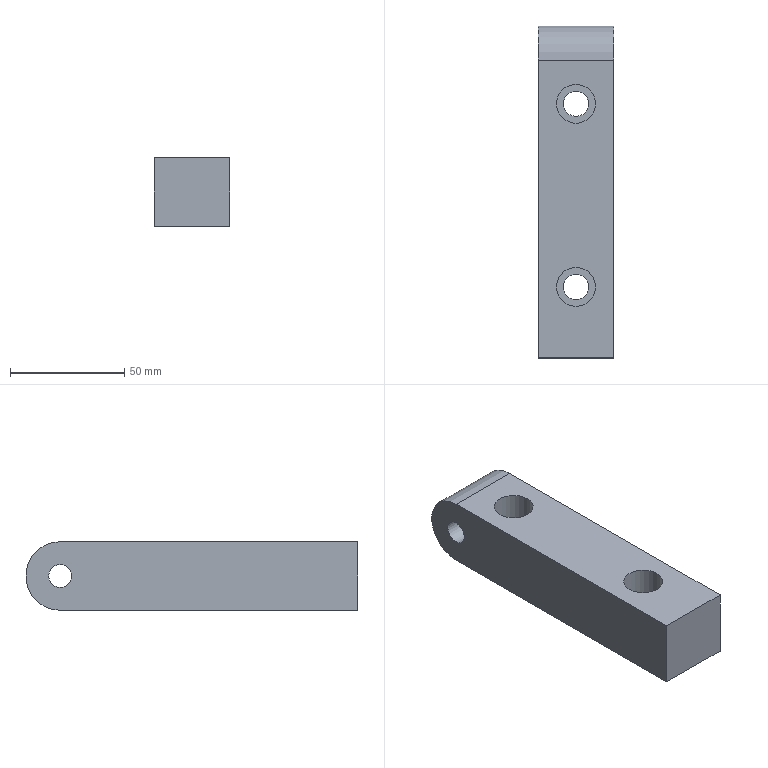Part | STEP file | gslz 2016.10.28-13_id1846_x_t | 1 solid | 13 faces | box 33 x 145.1 x 30 mm | volume 128184 mm3 | plane 7 | cylinder 6 | commonest cylinder face diameters 11 x2 17 x2 10.05 x1 30 x1
STEP:
#1=CARTESIAN_POINT('',(0.,0.,0.));
#2=DIRECTION('',(0.,0.,1.));
#3=DIRECTION('',(1.,0.,0.));
#4=AXIS2_PLACEMENT_3D('',#1,#2,#3);
#5=CARTESIAN_POINT('',(-1160.5,501.,-64.));
#6=VERTEX_POINT('',#5);
#7=CARTESIAN_POINT('',(-1171.5,501.,-64.));
#8=VERTEX_POINT('',#7);
#9=CARTESIAN_POINT('',(-1166.,501.,-64.));
#10=DIRECTION('',(0.,0.,1.));
#11=DIRECTION('',(-1.,0.,0.));
#12=AXIS2_PLACEMENT_3D('',#9,#10,#11);
#13=CIRCLE('',#12,5.5);
#14=CARTESIAN_POINT('',(-1166.,501.,-51.));
#15=DIRECTION('',(0.,0.,-1.));
#16=DIRECTION('',(0.,1.,0.));
#17=AXIS2_PLACEMENT_3D('',#14,#15,#16);
#18=CYLINDRICAL_SURFACE('',#17,5.5);
#19=CARTESIAN_POINT('',(10.996,13.));
#20=DIRECTION('',(-1.,0.));
#21=VECTOR('',#20,1.);
#22=LINE('',#19,#21);
#23=(GEOMETRIC_REPRESENTATION_CONTEXT(2)PARAMETRIC_REPRESENTATION_CONTEXT()REPRESENTATION_CONTEXT('',''));
#24=DEFINITIONAL_REPRESENTATION('',(#22),#23);
#25=PCURVE('',#18,#24);
#26=CARTESIAN_POINT('',(-1166.75,547.5,-64.));
#27=DIRECTION('',(0.,0.,1.));
#28=DIRECTION('',(-1.,0.,0.));
#29=AXIS2_PLACEMENT_3D('',#26,#27,#28);
#30=PLANE('',#29);
#31=CARTESIAN_POINT('',(-0.75,46.5));
#32=DIRECTION('',(1.,0.));
#33=AXIS2_PLACEMENT_2D('',#31,#32);
#34=CIRCLE('',#33,5.5);
#35=(GEOMETRIC_REPRESENTATION_CONTEXT(2)PARAMETRIC_REPRESENTATION_CONTEXT()REPRESENTATION_CONTEXT('',''));
#36=DEFINITIONAL_REPRESENTATION('',(#34),#35);
#37=PCURVE('',#30,#36);
#38=SURFACE_CURVE('',#13,(#25,#37),.PCURVE_S1.);
#39=EDGE_CURVE('',#6,#8,#38,.T.);
#40=ORIENTED_EDGE('',*,*,#39,.F.);
#41=CARTESIAN_POINT('',(-1160.5,501.,-79.));
#42=VERTEX_POINT('',#41);
#43=CARTESIAN_POINT('',(-1160.5,501.,-64.));
#44=CARTESIAN_POINT('',(-1160.5,501.,-79.));
#45=B_SPLINE_CURVE_WITH_KNOTS('',1,(#43,#44),.UNSPECIFIED.,.F.,.F.,(2,2),(13.,28.),.PIECEWISE_BEZIER_KNOTS.);
#46=CARTESIAN_POINT('',(7.854,0.));
#47=DIRECTION('',(0.,1.));
#48=VECTOR('',#47,1.);
#49=LINE('',#46,#48);
#50=(GEOMETRIC_REPRESENTATION_CONTEXT(2)PARAMETRIC_REPRESENTATION_CONTEXT()REPRESENTATION_CONTEXT('',''));
#51=DEFINITIONAL_REPRESENTATION('',(#49),#50);
#52=PCURVE('',#18,#51);
#53=CARTESIAN_POINT('',(1.571,0.));
#54=DIRECTION('',(0.,1.));
#55=VECTOR('',#54,1.);
#56=LINE('',#53,#55);
#57=(GEOMETRIC_REPRESENTATION_CONTEXT(2)PARAMETRIC_REPRESENTATION_CONTEXT()REPRESENTATION_CONTEXT('',''));
#58=DEFINITIONAL_REPRESENTATION('',(#56),#57);
#59=PCURVE('',#18,#58);
#60=SEAM_CURVE('',#45,(#52,#59),.PCURVE_S1.);
#61=EDGE_CURVE('',#6,#42,#60,.T.);
#62=ORIENTED_EDGE('',*,*,#61,.T.);
#63=CARTESIAN_POINT('',(-1166.,501.,-79.));
#64=DIRECTION('',(0.,0.,-1.));
#65=DIRECTION('',(1.,0.,0.));
#66=AXIS2_PLACEMENT_3D('',#63,#64,#65);
#67=CIRCLE('',#66,5.5);
#68=CARTESIAN_POINT('',(1.571,28.));
#69=DIRECTION('',(1.,0.));
#70=VECTOR('',#69,1.);
#71=LINE('',#68,#70);
#72=(GEOMETRIC_REPRESENTATION_CONTEXT(2)PARAMETRIC_REPRESENTATION_CONTEXT()REPRESENTATION_CONTEXT('',''));
#73=DEFINITIONAL_REPRESENTATION('',(#71),#72);
#74=PCURVE('',#18,#73);
#75=CARTESIAN_POINT('',(-1147.5,599.,-79.));
#76=DIRECTION('',(0.,0.,1.));
#77=DIRECTION('',(0.,-1.,0.));
#78=AXIS2_PLACEMENT_3D('',#75,#76,#77);
#79=PLANE('',#78);
#80=CARTESIAN_POINT('',(98.,-13.));
#81=CARTESIAN_POINT('',(107.526,-13.));
#82=CARTESIAN_POINT('',(102.763,-21.25));
#83=CARTESIAN_POINT('',(98.,-29.5));
#84=CARTESIAN_POINT('',(93.237,-21.25));
#85=CARTESIAN_POINT('',(88.474,-13.));
#86=CARTESIAN_POINT('',(98.,-13.));
#87=(BOUNDED_CURVE()B_SPLINE_CURVE(2,(#80,#81,#82,#83,#84,#85,#86),.UNSPECIFIED.,.T.,.F.)B_SPLINE_CURVE_WITH_KNOTS((1,2,2,2,2,1),(-2.094,0.,2.094,4.189,6.283,8.378),.UNSPECIFIED.)CURVE()GEOMETRIC_REPRESENTATION_ITEM()RATIONAL_B_SPLINE_CURVE((1.,0.5,1.,0.5,1.,0.5,1.))REPRESENTATION_ITEM(''));
#88=(GEOMETRIC_REPRESENTATION_CONTEXT(2)PARAMETRIC_REPRESENTATION_CONTEXT()REPRESENTATION_CONTEXT('',''));
#89=DEFINITIONAL_REPRESENTATION('',(#87),#88);
#90=PCURVE('',#79,#89);
#91=SURFACE_CURVE('',#67,(#74,#90),.PCURVE_S1.);
#92=EDGE_CURVE('',#42,#42,#91,.T.);
#93=ORIENTED_EDGE('',*,*,#92,.F.);
#94=ORIENTED_EDGE('',*,*,#61,.F.);
#95=CARTESIAN_POINT('',(-1166.,501.,-64.));
#96=DIRECTION('',(0.,0.,1.));
#97=DIRECTION('',(-1.,0.,0.));
#98=AXIS2_PLACEMENT_3D('',#95,#96,#97);
#99=CIRCLE('',#98,5.5);
#100=CARTESIAN_POINT('',(4.712,13.));
#101=DIRECTION('',(-1.,0.));
#102=VECTOR('',#101,1.);
#103=LINE('',#100,#102);
#104=(GEOMETRIC_REPRESENTATION_CONTEXT(2)PARAMETRIC_REPRESENTATION_CONTEXT()REPRESENTATION_CONTEXT('',''));
#105=DEFINITIONAL_REPRESENTATION('',(#103),#104);
#106=PCURVE('',#18,#105);
#107=CARTESIAN_POINT('',(-0.75,46.5));
#108=DIRECTION('',(1.,0.));
#109=AXIS2_PLACEMENT_2D('',#107,#108);
#110=CIRCLE('',#109,5.5);
#111=(GEOMETRIC_REPRESENTATION_CONTEXT(2)PARAMETRIC_REPRESENTATION_CONTEXT()REPRESENTATION_CONTEXT('',''));
#112=DEFINITIONAL_REPRESENTATION('',(#110),#111);
#113=PCURVE('',#30,#112);
#114=SURFACE_CURVE('',#99,(#106,#113),.PCURVE_S1.);
#115=EDGE_CURVE('',#8,#6,#114,.T.);
#116=ORIENTED_EDGE('',*,*,#115,.F.);
#117=EDGE_LOOP('',(#40,#62,#93,#94,#116));
#118=FACE_BOUND('',#117,.F.);
#119=ADVANCED_FACE('',(#118),#18,.F.);
#120=CARTESIAN_POINT('',(-1160.5,581.,-64.));
#121=VERTEX_POINT('',#120);
#122=CARTESIAN_POINT('',(-1171.5,581.,-64.));
#123=VERTEX_POINT('',#122);
#124=CARTESIAN_POINT('',(-1166.,581.,-64.));
#125=DIRECTION('',(0.,0.,1.));
#126=DIRECTION('',(-1.,0.,0.));
#127=AXIS2_PLACEMENT_3D('',#124,#125,#126);
#128=CIRCLE('',#127,5.5);
#129=CARTESIAN_POINT('',(-1166.,581.,-51.));
#130=DIRECTION('',(0.,0.,-1.));
#131=DIRECTION('',(0.,1.,0.));
#132=AXIS2_PLACEMENT_3D('',#129,#130,#131);
#133=CYLINDRICAL_SURFACE('',#132,5.5);
#134=CARTESIAN_POINT('',(10.996,13.));
#135=DIRECTION('',(-1.,0.));
#136=VECTOR('',#135,1.);
#137=LINE('',#134,#136);
#138=(GEOMETRIC_REPRESENTATION_CONTEXT(2)PARAMETRIC_REPRESENTATION_CONTEXT()REPRESENTATION_CONTEXT('',''));
#139=DEFINITIONAL_REPRESENTATION('',(#137),#138);
#140=PCURVE('',#133,#139);
#141=CARTESIAN_POINT('',(-1166.75,537.5,-64.));
#142=DIRECTION('',(0.,0.,1.));
#143=DIRECTION('',(-1.,0.,0.));
#144=AXIS2_PLACEMENT_3D('',#141,#142,#143);
#145=PLANE('',#144);
#146=CARTESIAN_POINT('',(-0.75,-43.5));
#147=DIRECTION('',(1.,0.));
#148=AXIS2_PLACEMENT_2D('',#146,#147);
#149=CIRCLE('',#148,5.5);
#150=(GEOMETRIC_REPRESENTATION_CONTEXT(2)PARAMETRIC_REPRESENTATION_CONTEXT()REPRESENTATION_CONTEXT('',''));
#151=DEFINITIONAL_REPRESENTATION('',(#149),#150);
#152=PCURVE('',#145,#151);
#153=SURFACE_CURVE('',#128,(#140,#152),.PCURVE_S1.);
#154=EDGE_CURVE('',#121,#123,#153,.T.);
#155=ORIENTED_EDGE('',*,*,#154,.F.);
#156=CARTESIAN_POINT('',(-1160.5,581.,-79.));
#157=VERTEX_POINT('',#156);
#158=CARTESIAN_POINT('',(-1160.5,581.,-64.));
#159=CARTESIAN_POINT('',(-1160.5,581.,-79.));
#160=B_SPLINE_CURVE_WITH_KNOTS('',1,(#158,#159),.UNSPECIFIED.,.F.,.F.,(2,2),(13.,28.),.PIECEWISE_BEZIER_KNOTS.);
#161=CARTESIAN_POINT('',(7.854,0.));
#162=DIRECTION('',(0.,1.));
#163=VECTOR('',#162,1.);
#164=LINE('',#161,#163);
#165=(GEOMETRIC_REPRESENTATION_CONTEXT(2)PARAMETRIC_REPRESENTATION_CONTEXT()REPRESENTATION_CONTEXT('',''));
#166=DEFINITIONAL_REPRESENTATION('',(#164),#165);
#167=PCURVE('',#133,#166);
#168=CARTESIAN_POINT('',(1.571,0.));
#169=DIRECTION('',(0.,1.));
#170=VECTOR('',#169,1.);
#171=LINE('',#168,#170);
#172=(GEOMETRIC_REPRESENTATION_CONTEXT(2)PARAMETRIC_REPRESENTATION_CONTEXT()REPRESENTATION_CONTEXT('',''));
#173=DEFINITIONAL_REPRESENTATION('',(#171),#172);
#174=PCURVE('',#133,#173);
#175=SEAM_CURVE('',#160,(#167,#174),.PCURVE_S1.);
#176=EDGE_CURVE('',#121,#157,#175,.T.);
#177=ORIENTED_EDGE('',*,*,#176,.T.);
#178=CARTESIAN_POINT('',(-1166.,581.,-79.));
#179=DIRECTION('',(0.,0.,-1.));
#180=DIRECTION('',(1.,0.,0.));
#181=AXIS2_PLACEMENT_3D('',#178,#179,#180);
#182=CIRCLE('',#181,5.5);
#183=CARTESIAN_POINT('',(1.571,28.));
#184=DIRECTION('',(1.,0.));
#185=VECTOR('',#184,1.);
#186=LINE('',#183,#185);
#187=(GEOMETRIC_REPRESENTATION_CONTEXT(2)PARAMETRIC_REPRESENTATION_CONTEXT()REPRESENTATION_CONTEXT('',''));
#188=DEFINITIONAL_REPRESENTATION('',(#186),#187);
#189=PCURVE('',#133,#188);
#190=CARTESIAN_POINT('',(18.,-13.));
#191=CARTESIAN_POINT('',(27.526,-13.));
#192=CARTESIAN_POINT('',(22.763,-21.25));
#193=CARTESIAN_POINT('',(18.,-29.5));
#194=CARTESIAN_POINT('',(13.237,-21.25));
#195=CARTESIAN_POINT('',(8.474,-13.));
#196=CARTESIAN_POINT('',(18.,-13.));
#197=(BOUNDED_CURVE()B_SPLINE_CURVE(2,(#190,#191,#192,#193,#194,#195,#196),.UNSPECIFIED.,.T.,.F.)B_SPLINE_CURVE_WITH_KNOTS((1,2,2,2,2,1),(-2.094,0.,2.094,4.189,6.283,8.378),.UNSPECIFIED.)CURVE()GEOMETRIC_REPRESENTATION_ITEM()RATIONAL_B_SPLINE_CURVE((1.,0.5,1.,0.5,1.,0.5,1.))REPRESENTATION_ITEM(''));
#198=(GEOMETRIC_REPRESENTATION_CONTEXT(2)PARAMETRIC_REPRESENTATION_CONTEXT()REPRESENTATION_CONTEXT('',''));
#199=DEFINITIONAL_REPRESENTATION('',(#197),#198);
#200=PCURVE('',#79,#199);
#201=SURFACE_CURVE('',#182,(#189,#200),.PCURVE_S1.);
#202=EDGE_CURVE('',#157,#157,#201,.T.);
#203=ORIENTED_EDGE('',*,*,#202,.F.);
#204=ORIENTED_EDGE('',*,*,#176,.F.);
#205=CARTESIAN_POINT('',(-1166.,581.,-64.));
#206=DIRECTION('',(0.,0.,1.));
#207=DIRECTION('',(-1.,0.,0.));
#208=AXIS2_PLACEMENT_3D('',#205,#206,#207);
#209=CIRCLE('',#208,5.5);
#210=CARTESIAN_POINT('',(4.712,13.));
#211=DIRECTION('',(-1.,0.));
#212=VECTOR('',#211,1.);
#213=LINE('',#210,#212);
#214=(GEOMETRIC_REPRESENTATION_CONTEXT(2)PARAMETRIC_REPRESENTATION_CONTEXT()REPRESENTATION_CONTEXT('',''));
#215=DEFINITIONAL_REPRESENTATION('',(#213),#214);
#216=PCURVE('',#133,#215);
#217=CARTESIAN_POINT('',(-0.75,-43.5));
#218=DIRECTION('',(1.,0.));
#219=AXIS2_PLACEMENT_2D('',#217,#218);
#220=CIRCLE('',#219,5.5);
#221=(GEOMETRIC_REPRESENTATION_CONTEXT(2)PARAMETRIC_REPRESENTATION_CONTEXT()REPRESENTATION_CONTEXT('',''));
#222=DEFINITIONAL_REPRESENTATION('',(#220),#221);
#223=PCURVE('',#145,#222);
#224=SURFACE_CURVE('',#209,(#216,#223),.PCURVE_S1.);
#225=EDGE_CURVE('',#123,#121,#224,.T.);
#226=ORIENTED_EDGE('',*,*,#225,.F.);
#227=EDGE_LOOP('',(#155,#177,#203,#204,#226));
#228=FACE_BOUND('',#227,.F.);
#229=ADVANCED_FACE('',(#228),#133,.F.);
#230=CARTESIAN_POINT('',(-1182.5,600.1,-69.025));
#231=VERTEX_POINT('',#230);
#232=CARTESIAN_POINT('',(-1182.5,600.1,-58.975));
#233=VERTEX_POINT('',#232);
#234=CARTESIAN_POINT('',(-1182.5,600.1,-64.));
#235=DIRECTION('',(1.,0.,0.));
#236=DIRECTION('',(0.,0.,-1.));
#237=AXIS2_PLACEMENT_3D('',#234,#235,#236);
#238=CIRCLE('',#237,5.025);
#239=CARTESIAN_POINT('',(-1182.5,599.25,-59.));
#240=DIRECTION('',(-1.,0.,0.));
#241=DIRECTION('',(0.,0.,-1.));
#242=AXIS2_PLACEMENT_3D('',#239,#240,#241);
#243=PLANE('',#242);
#244=CARTESIAN_POINT('',(10.025,-0.85));
#245=CARTESIAN_POINT('',(10.025,-9.554));
#246=CARTESIAN_POINT('',(2.488,-5.202));
#247=CARTESIAN_POINT('',(-5.05,-0.85));
#248=CARTESIAN_POINT('',(2.488,3.502));
#249=CARTESIAN_POINT('',(10.025,7.854));
#250=CARTESIAN_POINT('',(10.025,-0.85));
#251=(BOUNDED_CURVE()B_SPLINE_CURVE(2,(#244,#245,#246,#247,#248,#249,#250),.UNSPECIFIED.,.T.,.F.)B_SPLINE_CURVE_WITH_KNOTS((1,2,2,2,2,1),(-2.094,0.,2.094,4.189,6.283,8.378),.UNSPECIFIED.)CURVE()GEOMETRIC_REPRESENTATION_ITEM()RATIONAL_B_SPLINE_CURVE((1.,0.5,1.,0.5,1.,0.5,1.))REPRESENTATION_ITEM(''));
#252=(GEOMETRIC_REPRESENTATION_CONTEXT(2)PARAMETRIC_REPRESENTATION_CONTEXT()REPRESENTATION_CONTEXT('',''));
#253=DEFINITIONAL_REPRESENTATION('',(#251),#252);
#254=PCURVE('',#243,#253);
#255=CARTESIAN_POINT('',(-1262.5,600.1,-64.));
#256=DIRECTION('',(1.,0.,0.));
#257=DIRECTION('',(0.,1.,0.));
#258=AXIS2_PLACEMENT_3D('',#255,#256,#257);
#259=CYLINDRICAL_SURFACE('',#258,5.025);
#260=CARTESIAN_POINT('',(4.712,80.));
#261=DIRECTION('',(1.,0.));
#262=VECTOR('',#261,1.);
#263=LINE('',#260,#262);
#264=(GEOMETRIC_REPRESENTATION_CONTEXT(2)PARAMETRIC_REPRESENTATION_CONTEXT()REPRESENTATION_CONTEXT('',''));
#265=DEFINITIONAL_REPRESENTATION('',(#263),#264);
#266=PCURVE('',#259,#265);
#267=SURFACE_CURVE('',#238,(#254,#266),.PCURVE_S1.);
#268=EDGE_CURVE('',#231,#233,#267,.T.);
#269=ORIENTED_EDGE('',*,*,#268,.T.);
#270=CARTESIAN_POINT('',(-1182.5,600.1,-64.));
#271=DIRECTION('',(1.,0.,0.));
#272=DIRECTION('',(0.,0.,-1.));
#273=AXIS2_PLACEMENT_3D('',#270,#271,#272);
#274=CIRCLE('',#273,5.025);
#275=CARTESIAN_POINT('',(10.025,-0.85));
#276=CARTESIAN_POINT('',(10.025,-9.554));
#277=CARTESIAN_POINT('',(2.488,-5.202));
#278=CARTESIAN_POINT('',(-5.05,-0.85));
#279=CARTESIAN_POINT('',(2.488,3.502));
#280=CARTESIAN_POINT('',(10.025,7.854));
#281=CARTESIAN_POINT('',(10.025,-0.85));
#282=(BOUNDED_CURVE()B_SPLINE_CURVE(2,(#275,#276,#277,#278,#279,#280,#281),.UNSPECIFIED.,.T.,.F.)B_SPLINE_CURVE_WITH_KNOTS((1,2,2,2,2,1),(-2.094,0.,2.094,4.189,6.283,8.378),.UNSPECIFIED.)CURVE()GEOMETRIC_REPRESENTATION_ITEM()RATIONAL_B_SPLINE_CURVE((1.,0.5,1.,0.5,1.,0.5,1.))REPRESENTATION_ITEM(''));
#283=(GEOMETRIC_REPRESENTATION_CONTEXT(2)PARAMETRIC_REPRESENTATION_CONTEXT()REPRESENTATION_CONTEXT('',''));
#284=DEFINITIONAL_REPRESENTATION('',(#282),#283);
#285=PCURVE('',#243,#284);
#286=CARTESIAN_POINT('',(-1.571,80.));
#287=DIRECTION('',(1.,0.));
#288=VECTOR('',#287,1.);
#289=LINE('',#286,#288);
#290=(GEOMETRIC_REPRESENTATION_CONTEXT(2)PARAMETRIC_REPRESENTATION_CONTEXT()REPRESENTATION_CONTEXT('',''));
#291=DEFINITIONAL_REPRESENTATION('',(#289),#290);
#292=PCURVE('',#259,#291);
#293=SURFACE_CURVE('',#274,(#285,#292),.PCURVE_S1.);
#294=EDGE_CURVE('',#233,#231,#293,.T.);
#295=ORIENTED_EDGE('',*,*,#294,.T.);
#296=EDGE_LOOP('',(#269,#295));
#297=FACE_BOUND('',#296,.T.);
#298=CARTESIAN_POINT('',(-1182.5,600.1,-79.));
#299=VERTEX_POINT('',#298);
#300=CARTESIAN_POINT('',(-1182.5,470.,-79.));
#301=VERTEX_POINT('',#300);
#302=CARTESIAN_POINT('',(-1182.5,599.,-79.));
#303=DIRECTION('',(0.,-1.,0.));
#304=VECTOR('',#303,1.);
#305=LINE('',#302,#304);
#306=CARTESIAN_POINT('',(20.,0.25));
#307=DIRECTION('',(0.,1.));
#308=VECTOR('',#307,1.);
#309=LINE('',#306,#308);
#310=(GEOMETRIC_REPRESENTATION_CONTEXT(2)PARAMETRIC_REPRESENTATION_CONTEXT()REPRESENTATION_CONTEXT('',''));
#311=DEFINITIONAL_REPRESENTATION('',(#309),#310);
#312=PCURVE('',#243,#311);
#313=CARTESIAN_POINT('',(0.,-35.));
#314=DIRECTION('',(1.,0.));
#315=VECTOR('',#314,1.);
#316=LINE('',#313,#315);
#317=(GEOMETRIC_REPRESENTATION_CONTEXT(2)PARAMETRIC_REPRESENTATION_CONTEXT()REPRESENTATION_CONTEXT('',''));
#318=DEFINITIONAL_REPRESENTATION('',(#316),#317);
#319=PCURVE('',#79,#318);
#320=SURFACE_CURVE('',#305,(#312,#319),.PCURVE_S1.);
#321=EDGE_CURVE('',#299,#301,#320,.T.);
#322=ORIENTED_EDGE('',*,*,#321,.T.);
#323=CARTESIAN_POINT('',(-1182.5,470.,-49.));
#324=VERTEX_POINT('',#323);
#325=CARTESIAN_POINT('',(-1182.5,470.,-59.));
#326=DIRECTION('',(0.,0.,-1.));
#327=VECTOR('',#326,1.);
#328=LINE('',#325,#327);
#329=CARTESIAN_POINT('',(0.,129.25));
#330=DIRECTION('',(1.,0.));
#331=VECTOR('',#330,1.);
#332=LINE('',#329,#331);
#333=(GEOMETRIC_REPRESENTATION_CONTEXT(2)PARAMETRIC_REPRESENTATION_CONTEXT()REPRESENTATION_CONTEXT('',''));
#334=DEFINITIONAL_REPRESENTATION('',(#332),#333);
#335=PCURVE('',#243,#334);
#336=CARTESIAN_POINT('',(-1147.5,470.,-94.));
#337=DIRECTION('',(0.,1.,0.));
#338=DIRECTION('',(-1.,0.,0.));
#339=AXIS2_PLACEMENT_3D('',#336,#337,#338);
#340=PLANE('',#339);
#341=CARTESIAN_POINT('',(35.,35.));
#342=DIRECTION('',(0.,-1.));
#343=VECTOR('',#342,1.);
#344=LINE('',#341,#343);
#345=(GEOMETRIC_REPRESENTATION_CONTEXT(2)PARAMETRIC_REPRESENTATION_CONTEXT()REPRESENTATION_CONTEXT('',''));
#346=DEFINITIONAL_REPRESENTATION('',(#344),#345);
#347=PCURVE('',#340,#346);
#348=SURFACE_CURVE('',#328,(#335,#347),.PCURVE_S1.);
#349=EDGE_CURVE('',#324,#301,#348,.T.);
#350=ORIENTED_EDGE('',*,*,#349,.F.);
#351=CARTESIAN_POINT('',(-1182.5,600.1,-49.));
#352=VERTEX_POINT('',#351);
#353=CARTESIAN_POINT('',(-1182.5,619.,-49.));
#354=DIRECTION('',(0.,1.,0.));
#355=VECTOR('',#354,1.);
#356=LINE('',#353,#355);
#357=CARTESIAN_POINT('',(-10.,-19.75));
#358=DIRECTION('',(0.,-1.));
#359=VECTOR('',#358,1.);
#360=LINE('',#357,#359);
#361=(GEOMETRIC_REPRESENTATION_CONTEXT(2)PARAMETRIC_REPRESENTATION_CONTEXT()REPRESENTATION_CONTEXT('',''));
#362=DEFINITIONAL_REPRESENTATION('',(#360),#361);
#363=PCURVE('',#243,#362);
#364=CARTESIAN_POINT('',(-1147.5,619.,-49.));
#365=DIRECTION('',(0.,0.,-1.));
#366=DIRECTION('',(0.,1.,0.));
#367=AXIS2_PLACEMENT_3D('',#364,#365,#366);
#368=PLANE('',#367);
#369=CARTESIAN_POINT('',(0.,-35.));
#370=DIRECTION('',(1.,0.));
#371=VECTOR('',#370,1.);
#372=LINE('',#369,#371);
#373=(GEOMETRIC_REPRESENTATION_CONTEXT(2)PARAMETRIC_REPRESENTATION_CONTEXT()REPRESENTATION_CONTEXT('',''));
#374=DEFINITIONAL_REPRESENTATION('',(#372),#373);
#375=PCURVE('',#368,#374);
#376=SURFACE_CURVE('',#356,(#363,#375),.PCURVE_S1.);
#377=EDGE_CURVE('',#324,#352,#376,.T.);
#378=ORIENTED_EDGE('',*,*,#377,.T.);
#379=CARTESIAN_POINT('',(-1182.5,600.1,-64.));
#380=DIRECTION('',(-1.,0.,0.));
#381=DIRECTION('',(0.,0.,1.));
#382=AXIS2_PLACEMENT_3D('',#379,#380,#381);
#383=CIRCLE('',#382,15.);
#384=CARTESIAN_POINT('',(5.,-0.85));
#385=DIRECTION('',(-1.,0.));
#386=AXIS2_PLACEMENT_2D('',#384,#385);
#387=CIRCLE('',#386,15.);
#388=(GEOMETRIC_REPRESENTATION_CONTEXT(2)PARAMETRIC_REPRESENTATION_CONTEXT()REPRESENTATION_CONTEXT('',''));
#389=DEFINITIONAL_REPRESENTATION('',(#387),#388);
#390=PCURVE('',#243,#389);
#391=CARTESIAN_POINT('',(-1322.5,600.1,-64.));
#392=DIRECTION('',(1.,0.,0.));
#393=DIRECTION('',(0.,0.,-1.));
#394=AXIS2_PLACEMENT_3D('',#391,#392,#393);
#395=CYLINDRICAL_SURFACE('',#394,15.);
#396=CARTESIAN_POINT('',(3.142,140.));
#397=DIRECTION('',(-1.,0.));
#398=VECTOR('',#397,1.);
#399=LINE('',#396,#398);
#400=(GEOMETRIC_REPRESENTATION_CONTEXT(2)PARAMETRIC_REPRESENTATION_CONTEXT()REPRESENTATION_CONTEXT('',''));
#401=DEFINITIONAL_REPRESENTATION('',(#399),#400);
#402=PCURVE('',#395,#401);
#403=SURFACE_CURVE('',#383,(#390,#402),.PCURVE_S1.);
#404=EDGE_CURVE('',#352,#299,#403,.T.);
#405=ORIENTED_EDGE('',*,*,#404,.T.);
#406=EDGE_LOOP('',(#322,#350,#378,#405));
#407=FACE_BOUND('',#406,.T.);
#408=ADVANCED_FACE('',(#297,#407),#243,.T.);
#409=CARTESIAN_POINT('',(-1149.5,600.1,-58.975));
#410=VERTEX_POINT('',#409);
#411=CARTESIAN_POINT('',(-1149.5,600.1,-64.));
#412=DIRECTION('',(1.,0.,0.));
#413=DIRECTION('',(0.,0.,1.));
#414=AXIS2_PLACEMENT_3D('',#411,#412,#413);
#415=CIRCLE('',#414,5.025);
#416=CARTESIAN_POINT('',(-1149.5,615.,-67.));
#417=DIRECTION('',(1.,0.,0.));
#418=DIRECTION('',(0.,0.,-1.));
#419=AXIS2_PLACEMENT_3D('',#416,#417,#418);
#420=PLANE('',#419);
#421=CARTESIAN_POINT('',(-3.,-14.9));
#422=DIRECTION('',(-1.,0.));
#423=AXIS2_PLACEMENT_2D('',#421,#422);
#424=CIRCLE('',#423,5.025);
#425=(GEOMETRIC_REPRESENTATION_CONTEXT(2)PARAMETRIC_REPRESENTATION_CONTEXT()REPRESENTATION_CONTEXT('',''));
#426=DEFINITIONAL_REPRESENTATION('',(#424),#425);
#427=PCURVE('',#420,#426);
#428=CARTESIAN_POINT('',(1.571,113.));
#429=DIRECTION('',(1.,0.));
#430=VECTOR('',#429,1.);
#431=LINE('',#428,#430);
#432=(GEOMETRIC_REPRESENTATION_CONTEXT(2)PARAMETRIC_REPRESENTATION_CONTEXT()REPRESENTATION_CONTEXT('',''));
#433=DEFINITIONAL_REPRESENTATION('',(#431),#432);
#434=PCURVE('',#259,#433);
#435=SURFACE_CURVE('',#415,(#427,#434),.PCURVE_S1.);
#436=EDGE_CURVE('',#410,#410,#435,.T.);
#437=ORIENTED_EDGE('',*,*,#436,.F.);
#438=EDGE_LOOP('',(#437));
#439=FACE_BOUND('',#438,.T.);
#440=CARTESIAN_POINT('',(-1149.5,470.,-49.));
#441=VERTEX_POINT('',#440);
#442=CARTESIAN_POINT('',(-1149.5,470.,-79.));
#443=VERTEX_POINT('',#442);
#444=CARTESIAN_POINT('',(-1149.5,470.,-94.));
#445=DIRECTION('',(0.,0.,-1.));
#446=VECTOR('',#445,1.);
#447=LINE('',#444,#446);
#448=CARTESIAN_POINT('',(27.,-145.));
#449=DIRECTION('',(1.,0.));
#450=VECTOR('',#449,1.);
#451=LINE('',#448,#450);
#452=(GEOMETRIC_REPRESENTATION_CONTEXT(2)PARAMETRIC_REPRESENTATION_CONTEXT()REPRESENTATION_CONTEXT('',''));
#453=DEFINITIONAL_REPRESENTATION('',(#451),#452);
#454=PCURVE('',#420,#453);
#455=CARTESIAN_POINT('',(2.,0.));
#456=DIRECTION('',(0.,-1.));
#457=VECTOR('',#456,1.);
#458=LINE('',#455,#457);
#459=(GEOMETRIC_REPRESENTATION_CONTEXT(2)PARAMETRIC_REPRESENTATION_CONTEXT()REPRESENTATION_CONTEXT('',''));
#460=DEFINITIONAL_REPRESENTATION('',(#458),#459);
#461=PCURVE('',#340,#460);
#462=SURFACE_CURVE('',#447,(#454,#461),.PCURVE_S1.);
#463=EDGE_CURVE('',#441,#443,#462,.T.);
#464=ORIENTED_EDGE('',*,*,#463,.T.);
#465=CARTESIAN_POINT('',(-1149.5,600.1,-79.));
#466=VERTEX_POINT('',#465);
#467=CARTESIAN_POINT('',(-1149.5,615.,-79.));
#468=DIRECTION('',(0.,-1.,0.));
#469=VECTOR('',#468,1.);
#470=LINE('',#467,#469);
#471=CARTESIAN_POINT('',(12.,0.));
#472=DIRECTION('',(0.,-1.));
#473=VECTOR('',#472,1.);
#474=LINE('',#471,#473);
#475=(GEOMETRIC_REPRESENTATION_CONTEXT(2)PARAMETRIC_REPRESENTATION_CONTEXT()REPRESENTATION_CONTEXT('',''));
#476=DEFINITIONAL_REPRESENTATION('',(#474),#475);
#477=PCURVE('',#420,#476);
#478=CARTESIAN_POINT('',(-16.,-2.));
#479=DIRECTION('',(1.,0.));
#480=VECTOR('',#479,1.);
#481=LINE('',#478,#480);
#482=(GEOMETRIC_REPRESENTATION_CONTEXT(2)PARAMETRIC_REPRESENTATION_CONTEXT()REPRESENTATION_CONTEXT('',''));
#483=DEFINITIONAL_REPRESENTATION('',(#481),#482);
#484=PCURVE('',#79,#483);
#485=SURFACE_CURVE('',#470,(#477,#484),.PCURVE_S1.);
#486=EDGE_CURVE('',#466,#443,#485,.T.);
#487=ORIENTED_EDGE('',*,*,#486,.F.);
#488=CARTESIAN_POINT('',(-1149.5,600.1,-49.));
#489=VERTEX_POINT('',#488);
#490=CARTESIAN_POINT('',(-1149.5,600.1,-64.));
#491=DIRECTION('',(1.,0.,0.));
#492=DIRECTION('',(0.,0.,-1.));
#493=AXIS2_PLACEMENT_3D('',#490,#491,#492);
#494=CIRCLE('',#493,15.);
#495=CARTESIAN_POINT('',(-3.,-14.9));
#496=DIRECTION('',(1.,0.));
#497=AXIS2_PLACEMENT_2D('',#495,#496);
#498=CIRCLE('',#497,15.);
#499=(GEOMETRIC_REPRESENTATION_CONTEXT(2)PARAMETRIC_REPRESENTATION_CONTEXT()REPRESENTATION_CONTEXT('',''));
#500=DEFINITIONAL_REPRESENTATION('',(#498),#499);
#501=PCURVE('',#420,#500);
#502=CARTESIAN_POINT('',(0.,173.));
#503=DIRECTION('',(1.,0.));
#504=VECTOR('',#503,1.);
#505=LINE('',#502,#504);
#506=(GEOMETRIC_REPRESENTATION_CONTEXT(2)PARAMETRIC_REPRESENTATION_CONTEXT()REPRESENTATION_CONTEXT('',''));
#507=DEFINITIONAL_REPRESENTATION('',(#505),#506);
#508=PCURVE('',#395,#507);
#509=SURFACE_CURVE('',#494,(#501,#508),.PCURVE_S1.);
#510=EDGE_CURVE('',#466,#489,#509,.T.);
#511=ORIENTED_EDGE('',*,*,#510,.T.);
#512=CARTESIAN_POINT('',(-1149.5,615.,-49.));
#513=DIRECTION('',(0.,1.,0.));
#514=VECTOR('',#513,1.);
#515=LINE('',#512,#514);
#516=CARTESIAN_POINT('',(-18.,0.));
#517=DIRECTION('',(0.,1.));
#518=VECTOR('',#517,1.);
#519=LINE('',#516,#518);
#520=(GEOMETRIC_REPRESENTATION_CONTEXT(2)PARAMETRIC_REPRESENTATION_CONTEXT()REPRESENTATION_CONTEXT('',''));
#521=DEFINITIONAL_REPRESENTATION('',(#519),#520);
#522=PCURVE('',#420,#521);
#523=CARTESIAN_POINT('',(-4.,-2.));
#524=DIRECTION('',(1.,0.));
#525=VECTOR('',#524,1.);
#526=LINE('',#523,#525);
#527=(GEOMETRIC_REPRESENTATION_CONTEXT(2)PARAMETRIC_REPRESENTATION_CONTEXT()REPRESENTATION_CONTEXT('',''));
#528=DEFINITIONAL_REPRESENTATION('',(#526),#527);
#529=PCURVE('',#368,#528);
#530=SURFACE_CURVE('',#515,(#522,#529),.PCURVE_S1.);
#531=EDGE_CURVE('',#441,#489,#530,.T.);
#532=ORIENTED_EDGE('',*,*,#531,.F.);
#533=EDGE_LOOP('',(#464,#487,#511,#532));
#534=FACE_BOUND('',#533,.T.);
#535=ADVANCED_FACE('',(#439,#534),#420,.T.);
#536=CARTESIAN_POINT('',(-1147.5,470.,-79.));
#537=DIRECTION('',(-1.,0.,0.));
#538=VECTOR('',#537,1.);
#539=LINE('',#536,#538);
#540=CARTESIAN_POINT('',(0.,15.));
#541=DIRECTION('',(1.,0.));
#542=VECTOR('',#541,1.);
#543=LINE('',#540,#542);
#544=(GEOMETRIC_REPRESENTATION_CONTEXT(2)PARAMETRIC_REPRESENTATION_CONTEXT()REPRESENTATION_CONTEXT('',''));
#545=DEFINITIONAL_REPRESENTATION('',(#543),#544);
#546=PCURVE('',#340,#545);
#547=CARTESIAN_POINT('',(129.,0.));
#548=DIRECTION('',(0.,-1.));
#549=VECTOR('',#548,1.);
#550=LINE('',#547,#549);
#551=(GEOMETRIC_REPRESENTATION_CONTEXT(2)PARAMETRIC_REPRESENTATION_CONTEXT()REPRESENTATION_CONTEXT('',''));
#552=DEFINITIONAL_REPRESENTATION('',(#550),#551);
#553=PCURVE('',#79,#552);
#554=SURFACE_CURVE('',#539,(#546,#553),.PCURVE_S1.);
#555=EDGE_CURVE('',#443,#301,#554,.T.);
#556=ORIENTED_EDGE('',*,*,#555,.F.);
#557=ORIENTED_EDGE('',*,*,#463,.F.);
#558=CARTESIAN_POINT('',(-1147.5,470.,-49.));
#559=DIRECTION('',(-1.,0.,0.));
#560=VECTOR('',#559,1.);
#561=LINE('',#558,#560);
#562=CARTESIAN_POINT('',(0.,45.));
#563=DIRECTION('',(1.,0.));
#564=VECTOR('',#563,1.);
#565=LINE('',#562,#564);
#566=(GEOMETRIC_REPRESENTATION_CONTEXT(2)PARAMETRIC_REPRESENTATION_CONTEXT()REPRESENTATION_CONTEXT('',''));
#567=DEFINITIONAL_REPRESENTATION('',(#565),#566);
#568=PCURVE('',#340,#567);
#569=CARTESIAN_POINT('',(-149.,0.));
#570=DIRECTION('',(0.,-1.));
#571=VECTOR('',#570,1.);
#572=LINE('',#569,#571);
#573=(GEOMETRIC_REPRESENTATION_CONTEXT(2)PARAMETRIC_REPRESENTATION_CONTEXT()REPRESENTATION_CONTEXT('',''));
#574=DEFINITIONAL_REPRESENTATION('',(#572),#573);
#575=PCURVE('',#368,#574);
#576=SURFACE_CURVE('',#561,(#568,#575),.PCURVE_S1.);
#577=EDGE_CURVE('',#441,#324,#576,.T.);
#578=ORIENTED_EDGE('',*,*,#577,.T.);
#579=ORIENTED_EDGE('',*,*,#349,.T.);
#580=EDGE_LOOP('',(#556,#557,#578,#579));
#581=FACE_BOUND('',#580,.T.);
#582=ADVANCED_FACE('',(#581),#340,.F.);
#583=CARTESIAN_POINT('',(-1174.5,501.,-64.));
#584=VERTEX_POINT('',#583);
#585=CARTESIAN_POINT('',(-1166.,501.,-64.));
#586=DIRECTION('',(0.,0.,-1.));
#587=DIRECTION('',(-1.,0.,0.));
#588=AXIS2_PLACEMENT_3D('',#585,#586,#587);
#589=CIRCLE('',#588,8.5);
#590=CARTESIAN_POINT('',(7.75,46.5));
#591=CARTESIAN_POINT('',(7.75,31.778));
#592=CARTESIAN_POINT('',(-5.,39.139));
#593=CARTESIAN_POINT('',(-17.75,46.5));
#594=CARTESIAN_POINT('',(-5.,53.861));
#595=CARTESIAN_POINT('',(7.75,61.222));
#596=CARTESIAN_POINT('',(7.75,46.5));
#597=(BOUNDED_CURVE()B_SPLINE_CURVE(2,(#590,#591,#592,#593,#594,#595,#596),.UNSPECIFIED.,.T.,.F.)B_SPLINE_CURVE_WITH_KNOTS((1,2,2,2,2,1),(-2.094,0.,2.094,4.189,6.283,8.378),.UNSPECIFIED.)CURVE()GEOMETRIC_REPRESENTATION_ITEM()RATIONAL_B_SPLINE_CURVE((1.,0.5,1.,0.5,1.,0.5,1.))REPRESENTATION_ITEM(''));
#598=(GEOMETRIC_REPRESENTATION_CONTEXT(2)PARAMETRIC_REPRESENTATION_CONTEXT()REPRESENTATION_CONTEXT('',''));
#599=DEFINITIONAL_REPRESENTATION('',(#597),#598);
#600=PCURVE('',#30,#599);
#601=CARTESIAN_POINT('',(-1166.,501.,-51.));
#602=DIRECTION('',(0.,0.,-1.));
#603=DIRECTION('',(0.,1.,0.));
#604=AXIS2_PLACEMENT_3D('',#601,#602,#603);
#605=CYLINDRICAL_SURFACE('',#604,8.5);
#606=CARTESIAN_POINT('',(4.712,13.));
#607=DIRECTION('',(1.,0.));
#608=VECTOR('',#607,1.);
#609=LINE('',#606,#608);
#610=(GEOMETRIC_REPRESENTATION_CONTEXT(2)PARAMETRIC_REPRESENTATION_CONTEXT()REPRESENTATION_CONTEXT('',''));
#611=DEFINITIONAL_REPRESENTATION('',(#609),#610);
#612=PCURVE('',#605,#611);
#613=SURFACE_CURVE('',#589,(#600,#612),.PCURVE_S1.);
#614=EDGE_CURVE('',#584,#584,#613,.T.);
#615=ORIENTED_EDGE('',*,*,#614,.F.);
#616=EDGE_LOOP('',(#615));
#617=FACE_BOUND('',#616,.T.);
#618=ORIENTED_EDGE('',*,*,#115,.F.);
#619=ORIENTED_EDGE('',*,*,#39,.F.);
#620=EDGE_LOOP('',(#618,#619));
#621=FACE_BOUND('',#620,.T.);
#622=ADVANCED_FACE('',(#617,#621),#30,.T.);
#623=ORIENTED_EDGE('',*,*,#321,.F.);
#624=CARTESIAN_POINT('',(-1166.25,600.1,-79.));
#625=DIRECTION('',(1.,0.,0.));
#626=VECTOR('',#625,1.);
#627=LINE('',#624,#626);
#628=CARTESIAN_POINT('',(-1.1,-18.75));
#629=DIRECTION('',(0.,1.));
#630=VECTOR('',#629,1.);
#631=LINE('',#628,#630);
#632=(GEOMETRIC_REPRESENTATION_CONTEXT(2)PARAMETRIC_REPRESENTATION_CONTEXT()REPRESENTATION_CONTEXT('',''));
#633=DEFINITIONAL_REPRESENTATION('',(#631),#632);
#634=PCURVE('',#79,#633);
#635=CARTESIAN_POINT('',(0.,156.25));
#636=DIRECTION('',(0.,1.));
#637=VECTOR('',#636,1.);
#638=LINE('',#635,#637);
#639=(GEOMETRIC_REPRESENTATION_CONTEXT(2)PARAMETRIC_REPRESENTATION_CONTEXT()REPRESENTATION_CONTEXT('',''));
#640=DEFINITIONAL_REPRESENTATION('',(#638),#639);
#641=PCURVE('',#395,#640);
#642=SURFACE_CURVE('',#627,(#634,#641),.PCURVE_S1.);
#643=EDGE_CURVE('',#299,#466,#642,.T.);
#644=ORIENTED_EDGE('',*,*,#643,.T.);
#645=ORIENTED_EDGE('',*,*,#486,.T.);
#646=ORIENTED_EDGE('',*,*,#555,.T.);
#647=EDGE_LOOP('',(#623,#644,#645,#646));
#648=FACE_BOUND('',#647,.T.);
#649=ORIENTED_EDGE('',*,*,#92,.F.);
#650=EDGE_LOOP('',(#649));
#651=FACE_BOUND('',#650,.T.);
#652=ORIENTED_EDGE('',*,*,#202,.F.);
#653=EDGE_LOOP('',(#652));
#654=FACE_BOUND('',#653,.T.);
#655=ADVANCED_FACE('',(#648,#651,#654),#79,.F.);
#656=ORIENTED_EDGE('',*,*,#510,.F.);
#657=ORIENTED_EDGE('',*,*,#643,.F.);
#658=ORIENTED_EDGE('',*,*,#404,.F.);
#659=CARTESIAN_POINT('',(-1166.25,600.1,-49.));
#660=DIRECTION('',(-1.,0.,0.));
#661=VECTOR('',#660,1.);
#662=LINE('',#659,#661);
#663=CARTESIAN_POINT('',(3.142,156.25));
#664=DIRECTION('',(0.,-1.));
#665=VECTOR('',#664,1.);
#666=LINE('',#663,#665);
#667=(GEOMETRIC_REPRESENTATION_CONTEXT(2)PARAMETRIC_REPRESENTATION_CONTEXT()REPRESENTATION_CONTEXT('',''));
#668=DEFINITIONAL_REPRESENTATION('',(#666),#667);
#669=PCURVE('',#395,#668);
#670=CARTESIAN_POINT('',(-18.9,-18.75));
#671=DIRECTION('',(0.,-1.));
#672=VECTOR('',#671,1.);
#673=LINE('',#670,#672);
#674=(GEOMETRIC_REPRESENTATION_CONTEXT(2)PARAMETRIC_REPRESENTATION_CONTEXT()REPRESENTATION_CONTEXT('',''));
#675=DEFINITIONAL_REPRESENTATION('',(#673),#674);
#676=PCURVE('',#368,#675);
#677=SURFACE_CURVE('',#662,(#669,#676),.PCURVE_S1.);
#678=EDGE_CURVE('',#489,#352,#677,.T.);
#679=ORIENTED_EDGE('',*,*,#678,.F.);
#680=EDGE_LOOP('',(#656,#657,#658,#679));
#681=FACE_BOUND('',#680,.T.);
#682=ADVANCED_FACE('',(#681),#395,.T.);
#683=ORIENTED_EDGE('',*,*,#436,.F.);
#684=CARTESIAN_POINT('',(-1182.5,600.1,-58.975));
#685=CARTESIAN_POINT('',(-1149.5,600.1,-58.975));
#686=B_SPLINE_CURVE_WITH_KNOTS('',1,(#684,#685),.UNSPECIFIED.,.F.,.F.,(2,2),(80.,113.),.PIECEWISE_BEZIER_KNOTS.);
#687=CARTESIAN_POINT('',(1.571,0.));
#688=DIRECTION('',(0.,1.));
#689=VECTOR('',#688,1.);
#690=LINE('',#687,#689);
#691=(GEOMETRIC_REPRESENTATION_CONTEXT(2)PARAMETRIC_REPRESENTATION_CONTEXT()REPRESENTATION_CONTEXT('',''));
#692=DEFINITIONAL_REPRESENTATION('',(#690),#691);
#693=PCURVE('',#259,#692);
#694=CARTESIAN_POINT('',(7.854,0.));
#695=DIRECTION('',(0.,1.));
#696=VECTOR('',#695,1.);
#697=LINE('',#694,#696);
#698=(GEOMETRIC_REPRESENTATION_CONTEXT(2)PARAMETRIC_REPRESENTATION_CONTEXT()REPRESENTATION_CONTEXT('',''));
#699=DEFINITIONAL_REPRESENTATION('',(#697),#698);
#700=PCURVE('',#259,#699);
#701=SEAM_CURVE('',#686,(#693,#700),.PCURVE_S1.);
#702=EDGE_CURVE('',#233,#410,#701,.T.);
#703=ORIENTED_EDGE('',*,*,#702,.F.);
#704=ORIENTED_EDGE('',*,*,#294,.T.);
#705=ORIENTED_EDGE('',*,*,#268,.T.);
#706=ORIENTED_EDGE('',*,*,#702,.T.);
#707=EDGE_LOOP('',(#683,#703,#704,#705,#706));
#708=FACE_BOUND('',#707,.F.);
#709=ADVANCED_FACE('',(#708),#259,.F.);
#710=CARTESIAN_POINT('',(-1174.5,581.,-64.));
#711=VERTEX_POINT('',#710);
#712=CARTESIAN_POINT('',(-1166.,581.,-64.));
#713=DIRECTION('',(0.,0.,-1.));
#714=DIRECTION('',(-1.,0.,0.));
#715=AXIS2_PLACEMENT_3D('',#712,#713,#714);
#716=CIRCLE('',#715,8.5);
#717=CARTESIAN_POINT('',(7.75,-43.5));
#718=CARTESIAN_POINT('',(7.75,-58.222));
#719=CARTESIAN_POINT('',(-5.,-50.861));
#720=CARTESIAN_POINT('',(-17.75,-43.5));
#721=CARTESIAN_POINT('',(-5.,-36.139));
#722=CARTESIAN_POINT('',(7.75,-28.778));
#723=CARTESIAN_POINT('',(7.75,-43.5));
#724=(BOUNDED_CURVE()B_SPLINE_CURVE(2,(#717,#718,#719,#720,#721,#722,#723),.UNSPECIFIED.,.T.,.F.)B_SPLINE_CURVE_WITH_KNOTS((1,2,2,2,2,1),(-2.094,0.,2.094,4.189,6.283,8.378),.UNSPECIFIED.)CURVE()GEOMETRIC_REPRESENTATION_ITEM()RATIONAL_B_SPLINE_CURVE((1.,0.5,1.,0.5,1.,0.5,1.))REPRESENTATION_ITEM(''));
#725=(GEOMETRIC_REPRESENTATION_CONTEXT(2)PARAMETRIC_REPRESENTATION_CONTEXT()REPRESENTATION_CONTEXT('',''));
#726=DEFINITIONAL_REPRESENTATION('',(#724),#725);
#727=PCURVE('',#145,#726);
#728=CARTESIAN_POINT('',(-1166.,581.,-51.));
#729=DIRECTION('',(0.,0.,-1.));
#730=DIRECTION('',(0.,1.,0.));
#731=AXIS2_PLACEMENT_3D('',#728,#729,#730);
#732=CYLINDRICAL_SURFACE('',#731,8.5);
#733=CARTESIAN_POINT('',(4.712,13.));
#734=DIRECTION('',(1.,0.));
#735=VECTOR('',#734,1.);
#736=LINE('',#733,#735);
#737=(GEOMETRIC_REPRESENTATION_CONTEXT(2)PARAMETRIC_REPRESENTATION_CONTEXT()REPRESENTATION_CONTEXT('',''));
#738=DEFINITIONAL_REPRESENTATION('',(#736),#737);
#739=PCURVE('',#732,#738);
#740=SURFACE_CURVE('',#716,(#727,#739),.PCURVE_S1.);
#741=EDGE_CURVE('',#711,#711,#740,.T.);
#742=ORIENTED_EDGE('',*,*,#741,.F.);
#743=EDGE_LOOP('',(#742));
#744=FACE_BOUND('',#743,.T.);
#745=ORIENTED_EDGE('',*,*,#225,.F.);
#746=ORIENTED_EDGE('',*,*,#154,.F.);
#747=EDGE_LOOP('',(#745,#746));
#748=FACE_BOUND('',#747,.T.);
#749=ADVANCED_FACE('',(#744,#748),#145,.T.);
#750=ORIENTED_EDGE('',*,*,#531,.T.);
#751=ORIENTED_EDGE('',*,*,#678,.T.);
#752=ORIENTED_EDGE('',*,*,#377,.F.);
#753=ORIENTED_EDGE('',*,*,#577,.F.);
#754=EDGE_LOOP('',(#750,#751,#752,#753));
#755=FACE_BOUND('',#754,.T.);
#756=CARTESIAN_POINT('',(-1157.5,581.,-49.));
#757=VERTEX_POINT('',#756);
#758=CARTESIAN_POINT('',(-1174.5,581.,-49.));
#759=VERTEX_POINT('',#758);
#760=CARTESIAN_POINT('',(-1166.,581.,-49.));
#761=DIRECTION('',(0.,0.,-1.));
#762=DIRECTION('',(1.,0.,0.));
#763=AXIS2_PLACEMENT_3D('',#760,#761,#762);
#764=CIRCLE('',#763,8.5);
#765=CARTESIAN_POINT('',(-38.,-18.5));
#766=DIRECTION('',(0.,1.));
#767=AXIS2_PLACEMENT_2D('',#765,#766);
#768=CIRCLE('',#767,8.5);
#769=(GEOMETRIC_REPRESENTATION_CONTEXT(2)PARAMETRIC_REPRESENTATION_CONTEXT()REPRESENTATION_CONTEXT('',''));
#770=DEFINITIONAL_REPRESENTATION('',(#768),#769);
#771=PCURVE('',#368,#770);
#772=CARTESIAN_POINT('',(7.854,-2.));
#773=DIRECTION('',(1.,0.));
#774=VECTOR('',#773,1.);
#775=LINE('',#772,#774);
#776=(GEOMETRIC_REPRESENTATION_CONTEXT(2)PARAMETRIC_REPRESENTATION_CONTEXT()REPRESENTATION_CONTEXT('',''));
#777=DEFINITIONAL_REPRESENTATION('',(#775),#776);
#778=PCURVE('',#732,#777);
#779=SURFACE_CURVE('',#764,(#771,#778),.PCURVE_S1.);
#780=EDGE_CURVE('',#757,#759,#779,.T.);
#781=ORIENTED_EDGE('',*,*,#780,.T.);
#782=CARTESIAN_POINT('',(-1166.,581.,-49.));
#783=DIRECTION('',(0.,0.,-1.));
#784=DIRECTION('',(1.,0.,0.));
#785=AXIS2_PLACEMENT_3D('',#782,#783,#784);
#786=CIRCLE('',#785,8.5);
#787=CARTESIAN_POINT('',(-38.,-18.5));
#788=DIRECTION('',(0.,1.));
#789=AXIS2_PLACEMENT_2D('',#787,#788);
#790=CIRCLE('',#789,8.5);
#791=(GEOMETRIC_REPRESENTATION_CONTEXT(2)PARAMETRIC_REPRESENTATION_CONTEXT()REPRESENTATION_CONTEXT('',''));
#792=DEFINITIONAL_REPRESENTATION('',(#790),#791);
#793=PCURVE('',#368,#792);
#794=CARTESIAN_POINT('',(1.571,-2.));
#795=DIRECTION('',(1.,0.));
#796=VECTOR('',#795,1.);
#797=LINE('',#794,#796);
#798=(GEOMETRIC_REPRESENTATION_CONTEXT(2)PARAMETRIC_REPRESENTATION_CONTEXT()REPRESENTATION_CONTEXT('',''));
#799=DEFINITIONAL_REPRESENTATION('',(#797),#798);
#800=PCURVE('',#732,#799);
#801=SURFACE_CURVE('',#786,(#793,#800),.PCURVE_S1.);
#802=EDGE_CURVE('',#759,#757,#801,.T.);
#803=ORIENTED_EDGE('',*,*,#802,.T.);
#804=EDGE_LOOP('',(#781,#803));
#805=FACE_BOUND('',#804,.T.);
#806=CARTESIAN_POINT('',(-1157.5,501.,-49.));
#807=VERTEX_POINT('',#806);
#808=CARTESIAN_POINT('',(-1174.5,501.,-49.));
#809=VERTEX_POINT('',#808);
#810=CARTESIAN_POINT('',(-1166.,501.,-49.));
#811=DIRECTION('',(0.,0.,-1.));
#812=DIRECTION('',(1.,0.,0.));
#813=AXIS2_PLACEMENT_3D('',#810,#811,#812);
#814=CIRCLE('',#813,8.5);
#815=CARTESIAN_POINT('',(-118.,-18.5));
#816=DIRECTION('',(0.,1.));
#817=AXIS2_PLACEMENT_2D('',#815,#816);
#818=CIRCLE('',#817,8.5);
#819=(GEOMETRIC_REPRESENTATION_CONTEXT(2)PARAMETRIC_REPRESENTATION_CONTEXT()REPRESENTATION_CONTEXT('',''));
#820=DEFINITIONAL_REPRESENTATION('',(#818),#819);
#821=PCURVE('',#368,#820);
#822=CARTESIAN_POINT('',(7.854,-2.));
#823=DIRECTION('',(1.,0.));
#824=VECTOR('',#823,1.);
#825=LINE('',#822,#824);
#826=(GEOMETRIC_REPRESENTATION_CONTEXT(2)PARAMETRIC_REPRESENTATION_CONTEXT()REPRESENTATION_CONTEXT('',''));
#827=DEFINITIONAL_REPRESENTATION('',(#825),#826);
#828=PCURVE('',#605,#827);
#829=SURFACE_CURVE('',#814,(#821,#828),.PCURVE_S1.);
#830=EDGE_CURVE('',#807,#809,#829,.T.);
#831=ORIENTED_EDGE('',*,*,#830,.T.);
#832=CARTESIAN_POINT('',(-1166.,501.,-49.));
#833=DIRECTION('',(0.,0.,-1.));
#834=DIRECTION('',(1.,0.,0.));
#835=AXIS2_PLACEMENT_3D('',#832,#833,#834);
#836=CIRCLE('',#835,8.5);
#837=CARTESIAN_POINT('',(-118.,-18.5));
#838=DIRECTION('',(0.,1.));
#839=AXIS2_PLACEMENT_2D('',#837,#838);
#840=CIRCLE('',#839,8.5);
#841=(GEOMETRIC_REPRESENTATION_CONTEXT(2)PARAMETRIC_REPRESENTATION_CONTEXT()REPRESENTATION_CONTEXT('',''));
#842=DEFINITIONAL_REPRESENTATION('',(#840),#841);
#843=PCURVE('',#368,#842);
#844=CARTESIAN_POINT('',(1.571,-2.));
#845=DIRECTION('',(1.,0.));
#846=VECTOR('',#845,1.);
#847=LINE('',#844,#846);
#848=(GEOMETRIC_REPRESENTATION_CONTEXT(2)PARAMETRIC_REPRESENTATION_CONTEXT()REPRESENTATION_CONTEXT('',''));
#849=DEFINITIONAL_REPRESENTATION('',(#847),#848);
#850=PCURVE('',#605,#849);
#851=SURFACE_CURVE('',#836,(#843,#850),.PCURVE_S1.);
#852=EDGE_CURVE('',#809,#807,#851,.T.);
#853=ORIENTED_EDGE('',*,*,#852,.T.);
#854=EDGE_LOOP('',(#831,#853));
#855=FACE_BOUND('',#854,.T.);
#856=ADVANCED_FACE('',(#755,#805,#855),#368,.F.);
#857=ORIENTED_EDGE('',*,*,#614,.F.);
#858=CARTESIAN_POINT('',(-1174.5,501.,-49.));
#859=CARTESIAN_POINT('',(-1174.5,501.,-64.));
#860=B_SPLINE_CURVE_WITH_KNOTS('',1,(#858,#859),.UNSPECIFIED.,.F.,.F.,(2,2),(-2.,13.),.PIECEWISE_BEZIER_KNOTS.);
#861=CARTESIAN_POINT('',(4.712,0.));
#862=DIRECTION('',(0.,1.));
#863=VECTOR('',#862,1.);
#864=LINE('',#861,#863);
#865=(GEOMETRIC_REPRESENTATION_CONTEXT(2)PARAMETRIC_REPRESENTATION_CONTEXT()REPRESENTATION_CONTEXT('',''));
#866=DEFINITIONAL_REPRESENTATION('',(#864),#865);
#867=PCURVE('',#605,#866);
#868=CARTESIAN_POINT('',(10.996,0.));
#869=DIRECTION('',(0.,1.));
#870=VECTOR('',#869,1.);
#871=LINE('',#868,#870);
#872=(GEOMETRIC_REPRESENTATION_CONTEXT(2)PARAMETRIC_REPRESENTATION_CONTEXT()REPRESENTATION_CONTEXT('',''));
#873=DEFINITIONAL_REPRESENTATION('',(#871),#872);
#874=PCURVE('',#605,#873);
#875=SEAM_CURVE('',#860,(#867,#874),.PCURVE_S1.);
#876=EDGE_CURVE('',#809,#584,#875,.T.);
#877=ORIENTED_EDGE('',*,*,#876,.F.);
#878=ORIENTED_EDGE('',*,*,#852,.T.);
#879=ORIENTED_EDGE('',*,*,#830,.T.);
#880=ORIENTED_EDGE('',*,*,#876,.T.);
#881=EDGE_LOOP('',(#857,#877,#878,#879,#880));
#882=FACE_BOUND('',#881,.F.);
#883=ADVANCED_FACE('',(#882),#605,.F.);
#884=ORIENTED_EDGE('',*,*,#741,.F.);
#885=CARTESIAN_POINT('',(-1174.5,581.,-49.));
#886=CARTESIAN_POINT('',(-1174.5,581.,-64.));
#887=B_SPLINE_CURVE_WITH_KNOTS('',1,(#885,#886),.UNSPECIFIED.,.F.,.F.,(2,2),(-2.,13.),.PIECEWISE_BEZIER_KNOTS.);
#888=CARTESIAN_POINT('',(4.712,0.));
#889=DIRECTION('',(0.,1.));
#890=VECTOR('',#889,1.);
#891=LINE('',#888,#890);
#892=(GEOMETRIC_REPRESENTATION_CONTEXT(2)PARAMETRIC_REPRESENTATION_CONTEXT()REPRESENTATION_CONTEXT('',''));
#893=DEFINITIONAL_REPRESENTATION('',(#891),#892);
#894=PCURVE('',#732,#893);
#895=CARTESIAN_POINT('',(10.996,0.));
#896=DIRECTION('',(0.,1.));
#897=VECTOR('',#896,1.);
#898=LINE('',#895,#897);
#899=(GEOMETRIC_REPRESENTATION_CONTEXT(2)PARAMETRIC_REPRESENTATION_CONTEXT()REPRESENTATION_CONTEXT('',''));
#900=DEFINITIONAL_REPRESENTATION('',(#898),#899);
#901=PCURVE('',#732,#900);
#902=SEAM_CURVE('',#887,(#894,#901),.PCURVE_S1.);
#903=EDGE_CURVE('',#759,#711,#902,.T.);
#904=ORIENTED_EDGE('',*,*,#903,.F.);
#905=ORIENTED_EDGE('',*,*,#802,.T.);
#906=ORIENTED_EDGE('',*,*,#780,.T.);
#907=ORIENTED_EDGE('',*,*,#903,.T.);
#908=EDGE_LOOP('',(#884,#904,#905,#906,#907));
#909=FACE_BOUND('',#908,.F.);
#910=ADVANCED_FACE('',(#909),#732,.F.);
#911=CLOSED_SHELL('',(#119,#229,#408,#535,#582,#622,#655,#682,#709,#749,#856,#883,#910));
#912=MANIFOLD_SOLID_BREP('',#911);
#913=(LENGTH_UNIT()NAMED_UNIT(*)SI_UNIT(.MILLI.,.METRE.));
#914=UNCERTAINTY_MEASURE_WITH_UNIT(LENGTH_MEASURE(0.000005),#913,'','');
#915=(NAMED_UNIT(*)PLANE_ANGLE_UNIT()SI_UNIT($,.RADIAN.));
#916=(NAMED_UNIT(*)SI_UNIT($,.STERADIAN.)SOLID_ANGLE_UNIT());
#917=(GEOMETRIC_REPRESENTATION_CONTEXT(3)GLOBAL_UNCERTAINTY_ASSIGNED_CONTEXT((#914))GLOBAL_UNIT_ASSIGNED_CONTEXT((#913,#915,#916))REPRESENTATION_CONTEXT('',''));
#918=ADVANCED_BREP_SHAPE_REPRESENTATION('',(#4,#912),#917);